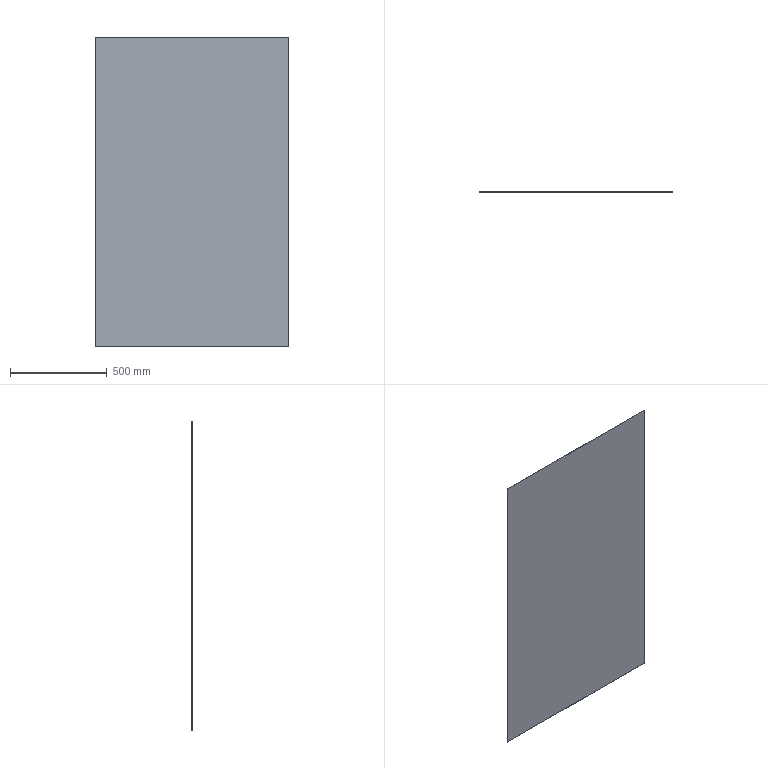Part | SolidWorks | features Extrusion 1 | 1 solid | 6 faces | box 1000 x 1 x 1601 mm | volume 1601000 mm3 | plane 6
STEP:
#1=CARTESIAN_POINT('',(500.,0.,800.5));
#2=VERTEX_POINT('',#1);
#3=CARTESIAN_POINT('',(500.,0.,-800.5));
#4=VERTEX_POINT('',#3);
#5=CARTESIAN_POINT('',(500.,0.,800.5));
#6=DIRECTION('',(0.,0.,-1.));
#7=VECTOR('',#6,1000.);
#8=LINE('',#5,#7);
#9=EDGE_CURVE('',#2,#4,#8,.T.);
#10=ORIENTED_EDGE('',*,*,#9,.T.);
#11=CARTESIAN_POINT('',(500.,1.,-800.5));
#12=VERTEX_POINT('',#11);
#13=CARTESIAN_POINT('',(500.,1.,-800.5));
#14=DIRECTION('',(0.,-1.,0.));
#15=VECTOR('',#14,1000.);
#16=LINE('',#13,#15);
#17=EDGE_CURVE('',#12,#4,#16,.T.);
#18=ORIENTED_EDGE('',*,*,#17,.F.);
#19=CARTESIAN_POINT('',(500.,1.,800.5));
#20=VERTEX_POINT('',#19);
#21=CARTESIAN_POINT('',(500.,1.,800.5));
#22=DIRECTION('',(0.,0.,-1.));
#23=VECTOR('',#22,1000.);
#24=LINE('',#21,#23);
#25=EDGE_CURVE('',#20,#12,#24,.T.);
#26=ORIENTED_EDGE('',*,*,#25,.F.);
#27=CARTESIAN_POINT('',(500.,1.,800.5));
#28=DIRECTION('',(0.,-1.,0.));
#29=VECTOR('',#28,1000.);
#30=LINE('',#27,#29);
#31=EDGE_CURVE('',#20,#2,#30,.T.);
#32=ORIENTED_EDGE('',*,*,#31,.T.);
#33=EDGE_LOOP('',(#10,#18,#26,#32));
#34=FACE_OUTER_BOUND('',#33,.T.);
#35=CARTESIAN_POINT('',(500.,1.,800.5));
#36=DIRECTION('',(-1.,0.,0.));
#37=DIRECTION('',(0.,0.,1.));
#38=AXIS2_PLACEMENT_3D('',#35,#36,#37);
#39=PLANE('',#38);
#40=ADVANCED_FACE('',(#34),#39,.F.);
#41=CARTESIAN_POINT('',(-500.,0.,-800.5));
#42=VERTEX_POINT('',#41);
#43=CARTESIAN_POINT('',(-500.,0.,-800.5));
#44=DIRECTION('',(-1.,0.,0.));
#45=VECTOR('',#44,1000.);
#46=LINE('',#43,#45);
#47=EDGE_CURVE('',#4,#42,#46,.T.);
#48=ORIENTED_EDGE('',*,*,#47,.T.);
#49=CARTESIAN_POINT('',(-500.,1.,-800.5));
#50=VERTEX_POINT('',#49);
#51=CARTESIAN_POINT('',(-500.,1.,-800.5));
#52=DIRECTION('',(0.,-1.,0.));
#53=VECTOR('',#52,1000.);
#54=LINE('',#51,#53);
#55=EDGE_CURVE('',#50,#42,#54,.T.);
#56=ORIENTED_EDGE('',*,*,#55,.F.);
#57=CARTESIAN_POINT('',(-500.,1.,-800.5));
#58=DIRECTION('',(-1.,0.,0.));
#59=VECTOR('',#58,1000.);
#60=LINE('',#57,#59);
#61=EDGE_CURVE('',#12,#50,#60,.T.);
#62=ORIENTED_EDGE('',*,*,#61,.F.);
#63=ORIENTED_EDGE('',*,*,#17,.T.);
#64=EDGE_LOOP('',(#48,#56,#62,#63));
#65=FACE_OUTER_BOUND('',#64,.T.);
#66=CARTESIAN_POINT('',(-500.,1.,-800.5));
#67=DIRECTION('',(0.,0.,1.));
#68=DIRECTION('',(1.,0.,0.));
#69=AXIS2_PLACEMENT_3D('',#66,#67,#68);
#70=PLANE('',#69);
#71=ADVANCED_FACE('',(#65),#70,.F.);
#72=CARTESIAN_POINT('',(-500.,0.,800.5));
#73=VERTEX_POINT('',#72);
#74=CARTESIAN_POINT('',(-500.,0.,800.5));
#75=DIRECTION('',(0.,0.,1.));
#76=VECTOR('',#75,1000.);
#77=LINE('',#74,#76);
#78=EDGE_CURVE('',#42,#73,#77,.T.);
#79=ORIENTED_EDGE('',*,*,#78,.T.);
#80=CARTESIAN_POINT('',(-500.,1.,800.5));
#81=VERTEX_POINT('',#80);
#82=CARTESIAN_POINT('',(-500.,1.,800.5));
#83=DIRECTION('',(0.,-1.,0.));
#84=VECTOR('',#83,1000.);
#85=LINE('',#82,#84);
#86=EDGE_CURVE('',#81,#73,#85,.T.);
#87=ORIENTED_EDGE('',*,*,#86,.F.);
#88=CARTESIAN_POINT('',(-500.,1.,800.5));
#89=DIRECTION('',(0.,0.,1.));
#90=VECTOR('',#89,1000.);
#91=LINE('',#88,#90);
#92=EDGE_CURVE('',#50,#81,#91,.T.);
#93=ORIENTED_EDGE('',*,*,#92,.F.);
#94=ORIENTED_EDGE('',*,*,#55,.T.);
#95=EDGE_LOOP('',(#79,#87,#93,#94));
#96=FACE_OUTER_BOUND('',#95,.T.);
#97=CARTESIAN_POINT('',(-500.,1.,800.5));
#98=DIRECTION('',(1.,0.,0.));
#99=DIRECTION('',(0.,0.,-1.));
#100=AXIS2_PLACEMENT_3D('',#97,#98,#99);
#101=PLANE('',#100);
#102=ADVANCED_FACE('',(#96),#101,.F.);
#103=CARTESIAN_POINT('',(-500.,0.,800.5));
#104=DIRECTION('',(1.,0.,0.));
#105=VECTOR('',#104,1000.);
#106=LINE('',#103,#105);
#107=EDGE_CURVE('',#73,#2,#106,.T.);
#108=ORIENTED_EDGE('',*,*,#107,.T.);
#109=ORIENTED_EDGE('',*,*,#31,.F.);
#110=CARTESIAN_POINT('',(-500.,1.,800.5));
#111=DIRECTION('',(1.,0.,0.));
#112=VECTOR('',#111,1000.);
#113=LINE('',#110,#112);
#114=EDGE_CURVE('',#81,#20,#113,.T.);
#115=ORIENTED_EDGE('',*,*,#114,.F.);
#116=ORIENTED_EDGE('',*,*,#86,.T.);
#117=EDGE_LOOP('',(#108,#109,#115,#116));
#118=FACE_OUTER_BOUND('',#117,.T.);
#119=CARTESIAN_POINT('',(-500.,1.,800.5));
#120=DIRECTION('',(0.,0.,-1.));
#121=DIRECTION('',(-1.,0.,0.));
#122=AXIS2_PLACEMENT_3D('',#119,#120,#121);
#123=PLANE('',#122);
#124=ADVANCED_FACE('',(#118),#123,.F.);
#125=ORIENTED_EDGE('',*,*,#25,.T.);
#126=ORIENTED_EDGE('',*,*,#61,.T.);
#127=ORIENTED_EDGE('',*,*,#92,.T.);
#128=ORIENTED_EDGE('',*,*,#114,.T.);
#129=EDGE_LOOP('',(#125,#126,#127,#128));
#130=FACE_OUTER_BOUND('',#129,.T.);
#131=CARTESIAN_POINT('',(0.,1.,0.));
#132=DIRECTION('',(0.,-1.,0.));
#133=DIRECTION('',(0.,0.,-1.));
#134=AXIS2_PLACEMENT_3D('',#131,#132,#133);
#135=PLANE('',#134);
#136=ADVANCED_FACE('',(#130),#135,.F.);
#137=ORIENTED_EDGE('',*,*,#9,.F.);
#138=ORIENTED_EDGE('',*,*,#107,.F.);
#139=ORIENTED_EDGE('',*,*,#78,.F.);
#140=ORIENTED_EDGE('',*,*,#47,.F.);
#141=EDGE_LOOP('',(#137,#138,#139,#140));
#142=FACE_OUTER_BOUND('',#141,.T.);
#143=CARTESIAN_POINT('',(0.,0.,0.));
#144=DIRECTION('',(0.,-1.,0.));
#145=DIRECTION('',(0.,0.,-1.));
#146=AXIS2_PLACEMENT_3D('',#143,#144,#145);
#147=PLANE('',#146);
#148=ADVANCED_FACE('',(#142),#147,.T.);
#149=CLOSED_SHELL('',(#40,#71,#102,#124,#136,#148));
#150=MANIFOLD_SOLID_BREP('',#149);
#151=CARTESIAN_POINT('',(0.,0.,0.));
#152=DIRECTION('',(0.,0.,1.));
#153=DIRECTION('',(1.,0.,0.));
#154=AXIS2_PLACEMENT_3D('',#151,#152,#153);
#155=(LENGTH_UNIT()NAMED_UNIT(*)SI_UNIT(.MILLI.,.METRE.));
#156=UNCERTAINTY_MEASURE_WITH_UNIT(LENGTH_MEASURE(0.00001),#155,'','');
#157=(NAMED_UNIT(*)PLANE_ANGLE_UNIT()SI_UNIT($,.RADIAN.));
#158=(NAMED_UNIT(*)SI_UNIT($,.STERADIAN.)SOLID_ANGLE_UNIT());
#159=(GEOMETRIC_REPRESENTATION_CONTEXT(3)GLOBAL_UNCERTAINTY_ASSIGNED_CONTEXT((#156))GLOBAL_UNIT_ASSIGNED_CONTEXT((#155,#157,#158))REPRESENTATION_CONTEXT('',''));
#160=ADVANCED_BREP_SHAPE_REPRESENTATION('',(#150,#154),#159);